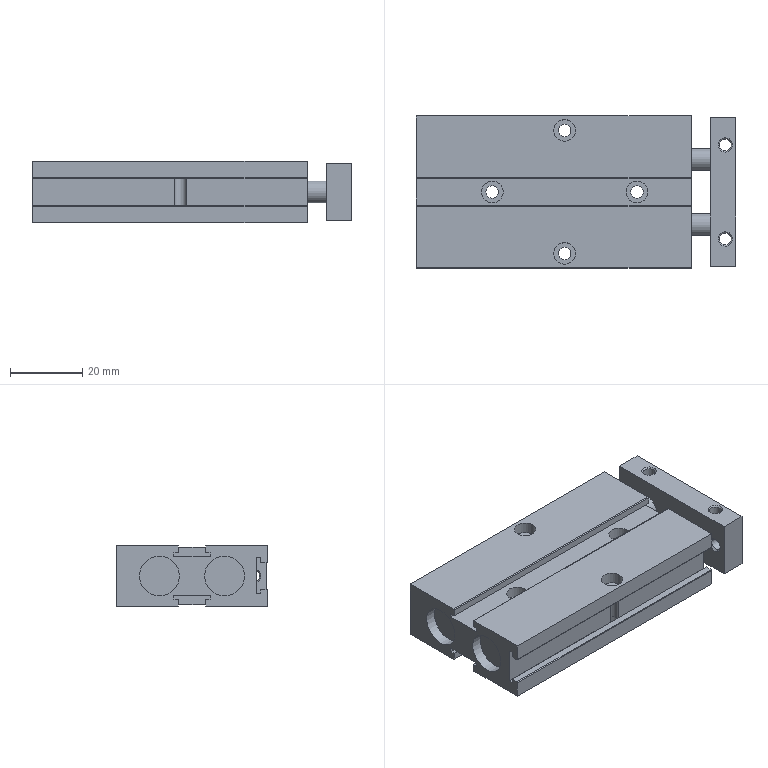Part | NX | features DATUM_CSYS 9, SKETCH 8, SIMPLE HOLE 6, SYMBOLIC_THREAD 4, EXTRUDE 3, HOLE PACKAGE 3, BREP 1 | 4 solids | 85 faces | box 88.3 x 42 x 17 mm | volume 51096 mm3 | plane 51 | cylinder 26 | cone 8 | commonest cylinder face diameters 6 x10 0.4 x6 3.3 x4 3.5 x4 11 x2